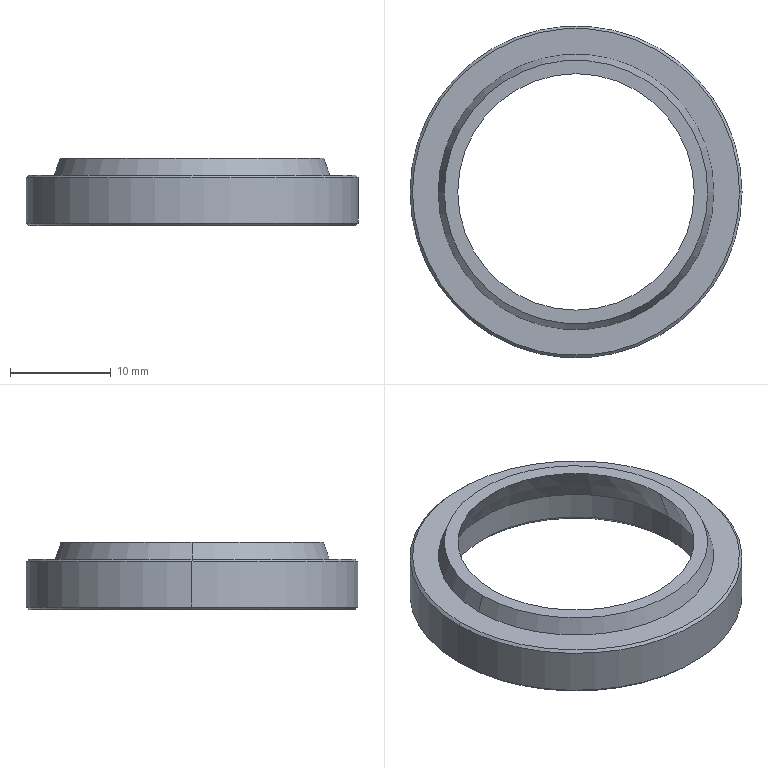Part | STEP file | Dust seal DHS25×33×4.5 | 1 solid | 17 faces | box 33 x 33 x 6.667 mm | volume 1830 mm3 | cone 10 | cylinder 4 | plane 3 | commonest cylinder face diameters 26 x2 33 x2
STEP:
#1=CARTESIAN_POINT('',(0.,0.,0.));
#2=DIRECTION('',(0.,0.,1.));
#3=DIRECTION('',(1.,0.,0.));
#4=AXIS2_PLACEMENT_3D('',#1,#2,#3);
#5=CARTESIAN_POINT('',(-16.25,0.,-6.667));
#6=VERTEX_POINT('',#5);
#7=CARTESIAN_POINT('',(16.25,0.,-6.667));
#8=VERTEX_POINT('',#7);
#9=CARTESIAN_POINT('',(0.,0.,-6.667));
#10=DIRECTION('',(0.,0.,-1.));
#11=DIRECTION('',(1.,0.,0.));
#12=AXIS2_PLACEMENT_3D('',#9,#10,#11);
#13=CIRCLE('',#12,16.25);
#14=CARTESIAN_POINT('',(0.,0.,-6.417));
#15=DIRECTION('',(0.,0.,1.));
#16=DIRECTION('',(1.,0.,0.));
#17=AXIS2_PLACEMENT_3D('',#14,#15,#16);
#18=CONICAL_SURFACE('',#17,16.5,0.7854);
#19=CARTESIAN_POINT('',(6.283,-0.25));
#20=DIRECTION('',(-1.,0.));
#21=VECTOR('',#20,1.);
#22=LINE('',#19,#21);
#23=(GEOMETRIC_REPRESENTATION_CONTEXT(2)PARAMETRIC_REPRESENTATION_CONTEXT()REPRESENTATION_CONTEXT('',''));
#24=DEFINITIONAL_REPRESENTATION('',(#22),#23);
#25=PCURVE('',#18,#24);
#26=CARTESIAN_POINT('',(-13.,0.,-6.667));
#27=DIRECTION('',(0.,0.,1.));
#28=DIRECTION('',(1.,0.,0.));
#29=AXIS2_PLACEMENT_3D('',#26,#27,#28);
#30=PLANE('',#29);
#31=CARTESIAN_POINT('',(29.25,0.));
#32=CARTESIAN_POINT('',(29.25,-28.146));
#33=CARTESIAN_POINT('',(4.875,-14.073));
#34=CARTESIAN_POINT('',(-19.5,0.));
#35=CARTESIAN_POINT('',(4.875,14.073));
#36=CARTESIAN_POINT('',(29.25,28.146));
#37=CARTESIAN_POINT('',(29.25,0.));
#38=(BOUNDED_CURVE()B_SPLINE_CURVE(2,(#31,#32,#33,#34,#35,#36,#37),.UNSPECIFIED.,.T.,.F.)B_SPLINE_CURVE_WITH_KNOTS((1,2,2,2,2,1),(-2.094,0.,2.094,4.189,6.283,8.378),.UNSPECIFIED.)CURVE()GEOMETRIC_REPRESENTATION_ITEM()RATIONAL_B_SPLINE_CURVE((1.,0.5,1.,0.5,1.,0.5,1.))REPRESENTATION_ITEM(''));
#39=(GEOMETRIC_REPRESENTATION_CONTEXT(2)PARAMETRIC_REPRESENTATION_CONTEXT()REPRESENTATION_CONTEXT('',''));
#40=DEFINITIONAL_REPRESENTATION('',(#38),#39);
#41=PCURVE('',#30,#40);
#42=SURFACE_CURVE('',#13,(#25,#41),.PCURVE_S1.);
#43=EDGE_CURVE('',#6,#8,#42,.T.);
#44=ORIENTED_EDGE('',*,*,#43,.F.);
#45=CARTESIAN_POINT('',(-16.5,0.,-6.417));
#46=VERTEX_POINT('',#45);
#47=CARTESIAN_POINT('',(-16.5,0.,-6.417));
#48=DIRECTION('',(-0.7071,0.,0.7071));
#49=VECTOR('',#48,1.);
#50=LINE('',#47,#49);
#51=CARTESIAN_POINT('',(3.142,0.));
#52=DIRECTION('',(0.,1.));
#53=VECTOR('',#52,1.);
#54=LINE('',#51,#53);
#55=(GEOMETRIC_REPRESENTATION_CONTEXT(2)PARAMETRIC_REPRESENTATION_CONTEXT()REPRESENTATION_CONTEXT('',''));
#56=DEFINITIONAL_REPRESENTATION('',(#54),#55);
#57=PCURVE('',#18,#56);
#58=CARTESIAN_POINT('',(0.,0.,-6.417));
#59=DIRECTION('',(0.,0.,1.));
#60=DIRECTION('',(1.,0.,0.));
#61=AXIS2_PLACEMENT_3D('',#58,#59,#60);
#62=CONICAL_SURFACE('',#61,16.5,0.7854);
#63=CARTESIAN_POINT('',(3.142,0.));
#64=DIRECTION('',(0.,1.));
#65=VECTOR('',#64,1.);
#66=LINE('',#63,#65);
#67=(GEOMETRIC_REPRESENTATION_CONTEXT(2)PARAMETRIC_REPRESENTATION_CONTEXT()REPRESENTATION_CONTEXT('',''));
#68=DEFINITIONAL_REPRESENTATION('',(#66),#67);
#69=PCURVE('',#62,#68);
#70=SURFACE_CURVE('',#50,(#57,#69),.PCURVE_S1.);
#71=EDGE_CURVE('',#6,#46,#70,.T.);
#72=ORIENTED_EDGE('',*,*,#71,.T.);
#73=CARTESIAN_POINT('',(16.5,0.,-6.417));
#74=VERTEX_POINT('',#73);
#75=CARTESIAN_POINT('',(0.,0.,-6.417));
#76=DIRECTION('',(0.,0.,1.));
#77=DIRECTION('',(1.,0.,0.));
#78=AXIS2_PLACEMENT_3D('',#75,#76,#77);
#79=CIRCLE('',#78,16.5);
#80=CARTESIAN_POINT('',(0.,0.));
#81=DIRECTION('',(1.,0.));
#82=VECTOR('',#81,1.);
#83=LINE('',#80,#82);
#84=(GEOMETRIC_REPRESENTATION_CONTEXT(2)PARAMETRIC_REPRESENTATION_CONTEXT()REPRESENTATION_CONTEXT('',''));
#85=DEFINITIONAL_REPRESENTATION('',(#83),#84);
#86=PCURVE('',#18,#85);
#87=CARTESIAN_POINT('',(0.,0.,9.196));
#88=DIRECTION('',(0.,0.,1.));
#89=DIRECTION('',(1.,0.,0.));
#90=AXIS2_PLACEMENT_3D('',#87,#88,#89);
#91=CYLINDRICAL_SURFACE('',#90,16.5);
#92=CARTESIAN_POINT('',(0.,-15.613));
#93=DIRECTION('',(1.,0.));
#94=VECTOR('',#93,1.);
#95=LINE('',#92,#94);
#96=(GEOMETRIC_REPRESENTATION_CONTEXT(2)PARAMETRIC_REPRESENTATION_CONTEXT()REPRESENTATION_CONTEXT('',''));
#97=DEFINITIONAL_REPRESENTATION('',(#95),#96);
#98=PCURVE('',#91,#97);
#99=SURFACE_CURVE('',#79,(#86,#98),.PCURVE_S1.);
#100=EDGE_CURVE('',#74,#46,#99,.T.);
#101=ORIENTED_EDGE('',*,*,#100,.F.);
#102=CARTESIAN_POINT('',(16.5,0.,-6.417));
#103=DIRECTION('',(0.7071,0.,0.7071));
#104=VECTOR('',#103,1.);
#105=LINE('',#102,#104);
#106=CARTESIAN_POINT('',(0.,0.));
#107=DIRECTION('',(0.,1.));
#108=VECTOR('',#107,1.);
#109=LINE('',#106,#108);
#110=(GEOMETRIC_REPRESENTATION_CONTEXT(2)PARAMETRIC_REPRESENTATION_CONTEXT()REPRESENTATION_CONTEXT('',''));
#111=DEFINITIONAL_REPRESENTATION('',(#109),#110);
#112=PCURVE('',#18,#111);
#113=CARTESIAN_POINT('',(6.283,0.));
#114=DIRECTION('',(0.,1.));
#115=VECTOR('',#114,1.);
#116=LINE('',#113,#115);
#117=(GEOMETRIC_REPRESENTATION_CONTEXT(2)PARAMETRIC_REPRESENTATION_CONTEXT()REPRESENTATION_CONTEXT('',''));
#118=DEFINITIONAL_REPRESENTATION('',(#116),#117);
#119=PCURVE('',#62,#118);
#120=SURFACE_CURVE('',#105,(#112,#119),.PCURVE_S1.);
#121=EDGE_CURVE('',#8,#74,#120,.T.);
#122=ORIENTED_EDGE('',*,*,#121,.F.);
#123=EDGE_LOOP('',(#44,#72,#101,#122));
#124=FACE_BOUND('',#123,.T.);
#125=ADVANCED_FACE('',(#124),#18,.T.);
#126=CARTESIAN_POINT('',(16.25,0.,-1.667));
#127=VERTEX_POINT('',#126);
#128=CARTESIAN_POINT('',(-16.25,0.,-1.667));
#129=VERTEX_POINT('',#128);
#130=CARTESIAN_POINT('',(0.,0.,-1.667));
#131=DIRECTION('',(0.,0.,1.));
#132=DIRECTION('',(-1.,0.,0.));
#133=AXIS2_PLACEMENT_3D('',#130,#131,#132);
#134=CIRCLE('',#133,16.25);
#135=CARTESIAN_POINT('',(0.,0.,-1.667));
#136=DIRECTION('',(0.,0.,-1.));
#137=DIRECTION('',(-1.,0.,0.));
#138=AXIS2_PLACEMENT_3D('',#135,#136,#137);
#139=CONICAL_SURFACE('',#138,16.25,0.7854);
#140=CARTESIAN_POINT('',(6.283,0.));
#141=DIRECTION('',(-1.,0.));
#142=VECTOR('',#141,1.);
#143=LINE('',#140,#142);
#144=(GEOMETRIC_REPRESENTATION_CONTEXT(2)PARAMETRIC_REPRESENTATION_CONTEXT()REPRESENTATION_CONTEXT('',''));
#145=DEFINITIONAL_REPRESENTATION('',(#143),#144);
#146=PCURVE('',#139,#145);
#147=CARTESIAN_POINT('',(-13.7,0.,-1.667));
#148=DIRECTION('',(0.,0.,-1.));
#149=DIRECTION('',(-1.,0.,0.));
#150=AXIS2_PLACEMENT_3D('',#147,#148,#149);
#151=PLANE('',#150);
#152=CARTESIAN_POINT('',(2.55,0.));
#153=CARTESIAN_POINT('',(2.55,-28.146));
#154=CARTESIAN_POINT('',(-21.825,-14.073));
#155=CARTESIAN_POINT('',(-46.2,0.));
#156=CARTESIAN_POINT('',(-21.825,14.073));
#157=CARTESIAN_POINT('',(2.55,28.146));
#158=CARTESIAN_POINT('',(2.55,0.));
#159=(BOUNDED_CURVE()B_SPLINE_CURVE(2,(#152,#153,#154,#155,#156,#157,#158),.UNSPECIFIED.,.T.,.F.)B_SPLINE_CURVE_WITH_KNOTS((1,2,2,2,2,1),(-2.094,0.,2.094,4.189,6.283,8.378),.UNSPECIFIED.)CURVE()GEOMETRIC_REPRESENTATION_ITEM()RATIONAL_B_SPLINE_CURVE((1.,0.5,1.,0.5,1.,0.5,1.))REPRESENTATION_ITEM(''));
#160=(GEOMETRIC_REPRESENTATION_CONTEXT(2)PARAMETRIC_REPRESENTATION_CONTEXT()REPRESENTATION_CONTEXT('',''));
#161=DEFINITIONAL_REPRESENTATION('',(#159),#160);
#162=PCURVE('',#151,#161);
#163=SURFACE_CURVE('',#134,(#146,#162),.PCURVE_S1.);
#164=EDGE_CURVE('',#127,#129,#163,.T.);
#165=ORIENTED_EDGE('',*,*,#164,.F.);
#166=CARTESIAN_POINT('',(16.5,0.,-1.917));
#167=VERTEX_POINT('',#166);
#168=CARTESIAN_POINT('',(16.25,0.,-1.667));
#169=DIRECTION('',(0.7071,0.,-0.7071));
#170=VECTOR('',#169,1.);
#171=LINE('',#168,#170);
#172=CARTESIAN_POINT('',(3.142,0.));
#173=DIRECTION('',(0.,1.));
#174=VECTOR('',#173,1.);
#175=LINE('',#172,#174);
#176=(GEOMETRIC_REPRESENTATION_CONTEXT(2)PARAMETRIC_REPRESENTATION_CONTEXT()REPRESENTATION_CONTEXT('',''));
#177=DEFINITIONAL_REPRESENTATION('',(#175),#176);
#178=PCURVE('',#139,#177);
#179=CARTESIAN_POINT('',(0.,0.,-1.667));
#180=DIRECTION('',(0.,0.,-1.));
#181=DIRECTION('',(-1.,0.,0.));
#182=AXIS2_PLACEMENT_3D('',#179,#180,#181);
#183=CONICAL_SURFACE('',#182,16.25,0.7854);
#184=CARTESIAN_POINT('',(3.142,0.));
#185=DIRECTION('',(0.,1.));
#186=VECTOR('',#185,1.);
#187=LINE('',#184,#186);
#188=(GEOMETRIC_REPRESENTATION_CONTEXT(2)PARAMETRIC_REPRESENTATION_CONTEXT()REPRESENTATION_CONTEXT('',''));
#189=DEFINITIONAL_REPRESENTATION('',(#187),#188);
#190=PCURVE('',#183,#189);
#191=SURFACE_CURVE('',#171,(#178,#190),.PCURVE_S1.);
#192=EDGE_CURVE('',#127,#167,#191,.T.);
#193=ORIENTED_EDGE('',*,*,#192,.T.);
#194=CARTESIAN_POINT('',(-16.5,0.,-1.917));
#195=VERTEX_POINT('',#194);
#196=CARTESIAN_POINT('',(0.,0.,-1.917));
#197=DIRECTION('',(0.,0.,-1.));
#198=DIRECTION('',(-1.,0.,0.));
#199=AXIS2_PLACEMENT_3D('',#196,#197,#198);
#200=CIRCLE('',#199,16.5);
#201=CARTESIAN_POINT('',(0.,0.25));
#202=DIRECTION('',(1.,0.));
#203=VECTOR('',#202,1.);
#204=LINE('',#201,#203);
#205=(GEOMETRIC_REPRESENTATION_CONTEXT(2)PARAMETRIC_REPRESENTATION_CONTEXT()REPRESENTATION_CONTEXT('',''));
#206=DEFINITIONAL_REPRESENTATION('',(#204),#205);
#207=PCURVE('',#139,#206);
#208=CARTESIAN_POINT('',(3.142,-11.113));
#209=DIRECTION('',(-1.,0.));
#210=VECTOR('',#209,1.);
#211=LINE('',#208,#210);
#212=(GEOMETRIC_REPRESENTATION_CONTEXT(2)PARAMETRIC_REPRESENTATION_CONTEXT()REPRESENTATION_CONTEXT('',''));
#213=DEFINITIONAL_REPRESENTATION('',(#211),#212);
#214=PCURVE('',#91,#213);
#215=SURFACE_CURVE('',#200,(#207,#214),.PCURVE_S1.);
#216=EDGE_CURVE('',#195,#167,#215,.T.);
#217=ORIENTED_EDGE('',*,*,#216,.F.);
#218=CARTESIAN_POINT('',(-16.25,0.,-1.667));
#219=DIRECTION('',(-0.7071,0.,-0.7071));
#220=VECTOR('',#219,1.);
#221=LINE('',#218,#220);
#222=CARTESIAN_POINT('',(0.,0.));
#223=DIRECTION('',(0.,1.));
#224=VECTOR('',#223,1.);
#225=LINE('',#222,#224);
#226=(GEOMETRIC_REPRESENTATION_CONTEXT(2)PARAMETRIC_REPRESENTATION_CONTEXT()REPRESENTATION_CONTEXT('',''));
#227=DEFINITIONAL_REPRESENTATION('',(#225),#226);
#228=PCURVE('',#139,#227);
#229=CARTESIAN_POINT('',(6.283,0.));
#230=DIRECTION('',(0.,1.));
#231=VECTOR('',#230,1.);
#232=LINE('',#229,#231);
#233=(GEOMETRIC_REPRESENTATION_CONTEXT(2)PARAMETRIC_REPRESENTATION_CONTEXT()REPRESENTATION_CONTEXT('',''));
#234=DEFINITIONAL_REPRESENTATION('',(#232),#233);
#235=PCURVE('',#183,#234);
#236=SURFACE_CURVE('',#221,(#228,#235),.PCURVE_S1.);
#237=EDGE_CURVE('',#129,#195,#236,.T.);
#238=ORIENTED_EDGE('',*,*,#237,.F.);
#239=EDGE_LOOP('',(#165,#193,#217,#238));
#240=FACE_BOUND('',#239,.T.);
#241=ADVANCED_FACE('',(#240),#139,.T.);
#242=CARTESIAN_POINT('',(-13.,0.,-6.167));
#243=VERTEX_POINT('',#242);
#244=CARTESIAN_POINT('',(-13.5,0.,-6.667));
#245=VERTEX_POINT('',#244);
#246=CARTESIAN_POINT('',(-13.5,0.,-6.667));
#247=DIRECTION('',(-0.7071,0.,-0.7071));
#248=VECTOR('',#247,1.);
#249=LINE('',#246,#248);
#250=CARTESIAN_POINT('',(0.,0.,-6.667));
#251=DIRECTION('',(0.,0.,-1.));
#252=DIRECTION('',(-1.,0.,0.));
#253=AXIS2_PLACEMENT_3D('',#250,#251,#252);
#254=CONICAL_SURFACE('',#253,13.5,0.7854);
#255=CARTESIAN_POINT('',(6.283,0.));
#256=DIRECTION('',(0.,1.));
#257=VECTOR('',#256,1.);
#258=LINE('',#255,#257);
#259=(GEOMETRIC_REPRESENTATION_CONTEXT(2)PARAMETRIC_REPRESENTATION_CONTEXT()REPRESENTATION_CONTEXT('',''));
#260=DEFINITIONAL_REPRESENTATION('',(#258),#259);
#261=PCURVE('',#254,#260);
#262=CARTESIAN_POINT('',(0.,0.,-6.667));
#263=DIRECTION('',(0.,0.,-1.));
#264=DIRECTION('',(-1.,0.,0.));
#265=AXIS2_PLACEMENT_3D('',#262,#263,#264);
#266=CONICAL_SURFACE('',#265,13.5,0.7854);
#267=CARTESIAN_POINT('',(0.,0.));
#268=DIRECTION('',(0.,1.));
#269=VECTOR('',#268,1.);
#270=LINE('',#267,#269);
#271=(GEOMETRIC_REPRESENTATION_CONTEXT(2)PARAMETRIC_REPRESENTATION_CONTEXT()REPRESENTATION_CONTEXT('',''));
#272=DEFINITIONAL_REPRESENTATION('',(#270),#271);
#273=PCURVE('',#266,#272);
#274=SURFACE_CURVE('',#249,(#261,#273),.PCURVE_S1.);
#275=EDGE_CURVE('',#243,#245,#274,.T.);
#276=ORIENTED_EDGE('',*,*,#275,.T.);
#277=CARTESIAN_POINT('',(13.5,0.,-6.667));
#278=VERTEX_POINT('',#277);
#279=CARTESIAN_POINT('',(0.,0.,-6.667));
#280=DIRECTION('',(0.,0.,1.));
#281=DIRECTION('',(1.,0.,0.));
#282=AXIS2_PLACEMENT_3D('',#279,#280,#281);
#283=CIRCLE('',#282,13.5);
#284=CARTESIAN_POINT('',(9.425,0.));
#285=DIRECTION('',(-1.,0.));
#286=VECTOR('',#285,1.);
#287=LINE('',#284,#286);
#288=(GEOMETRIC_REPRESENTATION_CONTEXT(2)PARAMETRIC_REPRESENTATION_CONTEXT()REPRESENTATION_CONTEXT('',''));
#289=DEFINITIONAL_REPRESENTATION('',(#287),#288);
#290=PCURVE('',#254,#289);
#291=CARTESIAN_POINT('',(13.,0.));
#292=DIRECTION('',(1.,0.));
#293=AXIS2_PLACEMENT_2D('',#291,#292);
#294=CIRCLE('',#293,13.5);
#295=(GEOMETRIC_REPRESENTATION_CONTEXT(2)PARAMETRIC_REPRESENTATION_CONTEXT()REPRESENTATION_CONTEXT('',''));
#296=DEFINITIONAL_REPRESENTATION('',(#294),#295);
#297=PCURVE('',#30,#296);
#298=SURFACE_CURVE('',#283,(#290,#297),.PCURVE_S1.);
#299=EDGE_CURVE('',#245,#278,#298,.T.);
#300=ORIENTED_EDGE('',*,*,#299,.T.);
#301=CARTESIAN_POINT('',(13.,0.,-6.167));
#302=VERTEX_POINT('',#301);
#303=CARTESIAN_POINT('',(13.5,0.,-6.667));
#304=DIRECTION('',(0.7071,0.,-0.7071));
#305=VECTOR('',#304,1.);
#306=LINE('',#303,#305);
#307=CARTESIAN_POINT('',(3.142,0.));
#308=DIRECTION('',(0.,1.));
#309=VECTOR('',#308,1.);
#310=LINE('',#307,#309);
#311=(GEOMETRIC_REPRESENTATION_CONTEXT(2)PARAMETRIC_REPRESENTATION_CONTEXT()REPRESENTATION_CONTEXT('',''));
#312=DEFINITIONAL_REPRESENTATION('',(#310),#311);
#313=PCURVE('',#254,#312);
#314=CARTESIAN_POINT('',(3.142,0.));
#315=DIRECTION('',(0.,1.));
#316=VECTOR('',#315,1.);
#317=LINE('',#314,#316);
#318=(GEOMETRIC_REPRESENTATION_CONTEXT(2)PARAMETRIC_REPRESENTATION_CONTEXT()REPRESENTATION_CONTEXT('',''));
#319=DEFINITIONAL_REPRESENTATION('',(#317),#318);
#320=PCURVE('',#266,#319);
#321=SURFACE_CURVE('',#306,(#313,#320),.PCURVE_S1.);
#322=EDGE_CURVE('',#302,#278,#321,.T.);
#323=ORIENTED_EDGE('',*,*,#322,.F.);
#324=CARTESIAN_POINT('',(0.,0.,-6.167));
#325=DIRECTION('',(0.,0.,-1.));
#326=DIRECTION('',(1.,0.,0.));
#327=AXIS2_PLACEMENT_3D('',#324,#325,#326);
#328=CIRCLE('',#327,13.);
#329=CARTESIAN_POINT('',(3.142,-0.5));
#330=DIRECTION('',(1.,0.));
#331=VECTOR('',#330,1.);
#332=LINE('',#329,#331);
#333=(GEOMETRIC_REPRESENTATION_CONTEXT(2)PARAMETRIC_REPRESENTATION_CONTEXT()REPRESENTATION_CONTEXT('',''));
#334=DEFINITIONAL_REPRESENTATION('',(#332),#333);
#335=PCURVE('',#254,#334);
#336=CARTESIAN_POINT('',(0.,0.,9.196));
#337=DIRECTION('',(0.,0.,1.));
#338=DIRECTION('',(1.,0.,0.));
#339=AXIS2_PLACEMENT_3D('',#336,#337,#338);
#340=CYLINDRICAL_SURFACE('',#339,13.);
#341=CARTESIAN_POINT('',(6.283,-15.363));
#342=DIRECTION('',(-1.,0.));
#343=VECTOR('',#342,1.);
#344=LINE('',#341,#343);
#345=(GEOMETRIC_REPRESENTATION_CONTEXT(2)PARAMETRIC_REPRESENTATION_CONTEXT()REPRESENTATION_CONTEXT('',''));
#346=DEFINITIONAL_REPRESENTATION('',(#344),#345);
#347=PCURVE('',#340,#346);
#348=SURFACE_CURVE('',#328,(#335,#347),.PCURVE_S1.);
#349=EDGE_CURVE('',#302,#243,#348,.T.);
#350=ORIENTED_EDGE('',*,*,#349,.T.);
#351=EDGE_LOOP('',(#276,#300,#323,#350));
#352=FACE_BOUND('',#351,.F.);
#353=ADVANCED_FACE('',(#352),#254,.F.);
#354=CARTESIAN_POINT('',(13.,0.,-3.434));
#355=VERTEX_POINT('',#354);
#356=CARTESIAN_POINT('',(13.,0.,9.196));
#357=DIRECTION('',(0.,0.,1.));
#358=VECTOR('',#357,1.);
#359=LINE('',#356,#358);
#360=CARTESIAN_POINT('',(6.283,0.));
#361=DIRECTION('',(0.,1.));
#362=VECTOR('',#361,1.);
#363=LINE('',#360,#362);
#364=(GEOMETRIC_REPRESENTATION_CONTEXT(2)PARAMETRIC_REPRESENTATION_CONTEXT()REPRESENTATION_CONTEXT('',''));
#365=DEFINITIONAL_REPRESENTATION('',(#363),#364);
#366=PCURVE('',#340,#365);
#367=CARTESIAN_POINT('',(0.,0.,9.196));
#368=DIRECTION('',(0.,0.,1.));
#369=DIRECTION('',(1.,0.,0.));
#370=AXIS2_PLACEMENT_3D('',#367,#368,#369);
#371=CYLINDRICAL_SURFACE('',#370,13.);
#372=CARTESIAN_POINT('',(0.,0.));
#373=DIRECTION('',(0.,1.));
#374=VECTOR('',#373,1.);
#375=LINE('',#372,#374);
#376=(GEOMETRIC_REPRESENTATION_CONTEXT(2)PARAMETRIC_REPRESENTATION_CONTEXT()REPRESENTATION_CONTEXT('',''));
#377=DEFINITIONAL_REPRESENTATION('',(#375),#376);
#378=PCURVE('',#371,#377);
#379=SURFACE_CURVE('',#359,(#366,#378),.PCURVE_S1.);
#380=EDGE_CURVE('',#302,#355,#379,.T.);
#381=ORIENTED_EDGE('',*,*,#380,.T.);
#382=CARTESIAN_POINT('',(-13.,0.,-3.434));
#383=VERTEX_POINT('',#382);
#384=CARTESIAN_POINT('',(0.,0.,-3.434));
#385=DIRECTION('',(0.,0.,1.));
#386=DIRECTION('',(1.,0.,0.));
#387=AXIS2_PLACEMENT_3D('',#384,#385,#386);
#388=CIRCLE('',#387,13.);
#389=CARTESIAN_POINT('',(0.,-12.63));
#390=DIRECTION('',(1.,0.));
#391=VECTOR('',#390,1.);
#392=LINE('',#389,#391);
#393=(GEOMETRIC_REPRESENTATION_CONTEXT(2)PARAMETRIC_REPRESENTATION_CONTEXT()REPRESENTATION_CONTEXT('',''));
#394=DEFINITIONAL_REPRESENTATION('',(#392),#393);
#395=PCURVE('',#340,#394);
#396=CARTESIAN_POINT('',(0.,0.,0.));
#397=DIRECTION('',(0.,0.,-1.));
#398=DIRECTION('',(-1.,0.,0.));
#399=AXIS2_PLACEMENT_3D('',#396,#397,#398);
#400=CONICAL_SURFACE('',#399,11.75,0.3491);
#401=CARTESIAN_POINT('',(9.425,3.434));
#402=DIRECTION('',(-1.,0.));
#403=VECTOR('',#402,1.);
#404=LINE('',#401,#403);
#405=(GEOMETRIC_REPRESENTATION_CONTEXT(2)PARAMETRIC_REPRESENTATION_CONTEXT()REPRESENTATION_CONTEXT('',''));
#406=DEFINITIONAL_REPRESENTATION('',(#404),#405);
#407=PCURVE('',#400,#406);
#408=SURFACE_CURVE('',#388,(#395,#407),.PCURVE_S1.);
#409=EDGE_CURVE('',#383,#355,#408,.T.);
#410=ORIENTED_EDGE('',*,*,#409,.F.);
#411=CARTESIAN_POINT('',(-13.,0.,9.196));
#412=DIRECTION('',(0.,0.,1.));
#413=VECTOR('',#412,1.);
#414=LINE('',#411,#413);
#415=CARTESIAN_POINT('',(3.142,0.));
#416=DIRECTION('',(0.,1.));
#417=VECTOR('',#416,1.);
#418=LINE('',#415,#417);
#419=(GEOMETRIC_REPRESENTATION_CONTEXT(2)PARAMETRIC_REPRESENTATION_CONTEXT()REPRESENTATION_CONTEXT('',''));
#420=DEFINITIONAL_REPRESENTATION('',(#418),#419);
#421=PCURVE('',#340,#420);
#422=CARTESIAN_POINT('',(3.142,0.));
#423=DIRECTION('',(0.,1.));
#424=VECTOR('',#423,1.);
#425=LINE('',#422,#424);
#426=(GEOMETRIC_REPRESENTATION_CONTEXT(2)PARAMETRIC_REPRESENTATION_CONTEXT()REPRESENTATION_CONTEXT('',''));
#427=DEFINITIONAL_REPRESENTATION('',(#425),#426);
#428=PCURVE('',#371,#427);
#429=SURFACE_CURVE('',#414,(#421,#428),.PCURVE_S1.);
#430=EDGE_CURVE('',#243,#383,#429,.T.);
#431=ORIENTED_EDGE('',*,*,#430,.F.);
#432=ORIENTED_EDGE('',*,*,#349,.F.);
#433=EDGE_LOOP('',(#381,#410,#431,#432));
#434=FACE_BOUND('',#433,.F.);
#435=ADVANCED_FACE('',(#434),#340,.F.);
#436=CARTESIAN_POINT('',(-11.75,0.,0.));
#437=VERTEX_POINT('',#436);
#438=CARTESIAN_POINT('',(-11.75,0.,0.));
#439=DIRECTION('',(-0.342,0.,-0.9397));
#440=VECTOR('',#439,1.);
#441=LINE('',#438,#440);
#442=CARTESIAN_POINT('',(6.283,0.));
#443=DIRECTION('',(0.,1.));
#444=VECTOR('',#443,1.);
#445=LINE('',#442,#444);
#446=(GEOMETRIC_REPRESENTATION_CONTEXT(2)PARAMETRIC_REPRESENTATION_CONTEXT()REPRESENTATION_CONTEXT('',''));
#447=DEFINITIONAL_REPRESENTATION('',(#445),#446);
#448=PCURVE('',#400,#447);
#449=CARTESIAN_POINT('',(0.,0.,0.));
#450=DIRECTION('',(0.,0.,-1.));
#451=DIRECTION('',(-1.,0.,0.));
#452=AXIS2_PLACEMENT_3D('',#449,#450,#451);
#453=CONICAL_SURFACE('',#452,11.75,0.3491);
#454=CARTESIAN_POINT('',(0.,0.));
#455=DIRECTION('',(0.,1.));
#456=VECTOR('',#455,1.);
#457=LINE('',#454,#456);
#458=(GEOMETRIC_REPRESENTATION_CONTEXT(2)PARAMETRIC_REPRESENTATION_CONTEXT()REPRESENTATION_CONTEXT('',''));
#459=DEFINITIONAL_REPRESENTATION('',(#457),#458);
#460=PCURVE('',#453,#459);
#461=SURFACE_CURVE('',#441,(#448,#460),.PCURVE_S1.);
#462=EDGE_CURVE('',#437,#383,#461,.T.);
#463=ORIENTED_EDGE('',*,*,#462,.T.);
#464=ORIENTED_EDGE('',*,*,#409,.T.);
#465=CARTESIAN_POINT('',(11.75,0.,0.));
#466=VERTEX_POINT('',#465);
#467=CARTESIAN_POINT('',(11.75,0.,0.));
#468=DIRECTION('',(0.342,0.,-0.9397));
#469=VECTOR('',#468,1.);
#470=LINE('',#467,#469);
#471=CARTESIAN_POINT('',(3.142,0.));
#472=DIRECTION('',(0.,1.));
#473=VECTOR('',#472,1.);
#474=LINE('',#471,#473);
#475=(GEOMETRIC_REPRESENTATION_CONTEXT(2)PARAMETRIC_REPRESENTATION_CONTEXT()REPRESENTATION_CONTEXT('',''));
#476=DEFINITIONAL_REPRESENTATION('',(#474),#475);
#477=PCURVE('',#400,#476);
#478=CARTESIAN_POINT('',(3.142,0.));
#479=DIRECTION('',(0.,1.));
#480=VECTOR('',#479,1.);
#481=LINE('',#478,#480);
#482=(GEOMETRIC_REPRESENTATION_CONTEXT(2)PARAMETRIC_REPRESENTATION_CONTEXT()REPRESENTATION_CONTEXT('',''));
#483=DEFINITIONAL_REPRESENTATION('',(#481),#482);
#484=PCURVE('',#453,#483);
#485=SURFACE_CURVE('',#470,(#477,#484),.PCURVE_S1.);
#486=EDGE_CURVE('',#466,#355,#485,.T.);
#487=ORIENTED_EDGE('',*,*,#486,.F.);
#488=CARTESIAN_POINT('',(0.,0.,0.));
#489=DIRECTION('',(0.,0.,1.));
#490=DIRECTION('',(1.,0.,0.));
#491=AXIS2_PLACEMENT_3D('',#488,#489,#490);
#492=CIRCLE('',#491,11.75);
#493=CARTESIAN_POINT('',(9.425,0.));
#494=DIRECTION('',(-1.,0.));
#495=VECTOR('',#494,1.);
#496=LINE('',#493,#495);
#497=(GEOMETRIC_REPRESENTATION_CONTEXT(2)PARAMETRIC_REPRESENTATION_CONTEXT()REPRESENTATION_CONTEXT('',''));
#498=DEFINITIONAL_REPRESENTATION('',(#496),#497);
#499=PCURVE('',#400,#498);
#500=CARTESIAN_POINT('',(-11.75,0.,0.));
#501=DIRECTION('',(0.,0.,-1.));
#502=DIRECTION('',(-1.,0.,0.));
#503=AXIS2_PLACEMENT_3D('',#500,#501,#502);
#504=PLANE('',#503);
#505=CARTESIAN_POINT('',(-23.5,0.));
#506=CARTESIAN_POINT('',(-23.5,20.352));
#507=CARTESIAN_POINT('',(-5.875,10.176));
#508=CARTESIAN_POINT('',(11.75,0.));
#509=CARTESIAN_POINT('',(-5.875,-10.176));
#510=CARTESIAN_POINT('',(-23.5,-20.352));
#511=CARTESIAN_POINT('',(-23.5,0.));
#512=(BOUNDED_CURVE()B_SPLINE_CURVE(2,(#505,#506,#507,#508,#509,#510,#511),.UNSPECIFIED.,.T.,.F.)B_SPLINE_CURVE_WITH_KNOTS((1,2,2,2,2,1),(-2.094,0.,2.094,4.189,6.283,8.378),.UNSPECIFIED.)CURVE()GEOMETRIC_REPRESENTATION_ITEM()RATIONAL_B_SPLINE_CURVE((1.,0.5,1.,0.5,1.,0.5,1.))REPRESENTATION_ITEM(''));
#513=(GEOMETRIC_REPRESENTATION_CONTEXT(2)PARAMETRIC_REPRESENTATION_CONTEXT()REPRESENTATION_CONTEXT('',''));
#514=DEFINITIONAL_REPRESENTATION('',(#512),#513);
#515=PCURVE('',#504,#514);
#516=SURFACE_CURVE('',#492,(#499,#515),.PCURVE_S1.);
#517=EDGE_CURVE('',#437,#466,#516,.T.);
#518=ORIENTED_EDGE('',*,*,#517,.F.);
#519=EDGE_LOOP('',(#463,#464,#487,#518));
#520=FACE_BOUND('',#519,.F.);
#521=ADVANCED_FACE('',(#520),#400,.F.);
#522=CARTESIAN_POINT('',(13.093,0.,0.));
#523=VERTEX_POINT('',#522);
#524=CARTESIAN_POINT('',(-13.093,0.,0.));
#525=VERTEX_POINT('',#524);
#526=CARTESIAN_POINT('',(0.,0.,0.));
#527=DIRECTION('',(0.,0.,1.));
#528=DIRECTION('',(1.,0.,0.));
#529=AXIS2_PLACEMENT_3D('',#526,#527,#528);
#530=CIRCLE('',#529,13.093);
#531=CARTESIAN_POINT('',(0.,0.,-1.667));
#532=DIRECTION('',(0.,0.,-1.));
#533=DIRECTION('',(-1.,0.,0.));
#534=AXIS2_PLACEMENT_3D('',#531,#532,#533);
#535=CONICAL_SURFACE('',#534,13.7,0.3491);
#536=CARTESIAN_POINT('',(3.142,-1.667));
#537=DIRECTION('',(-1.,0.));
#538=VECTOR('',#537,1.);
#539=LINE('',#536,#538);
#540=(GEOMETRIC_REPRESENTATION_CONTEXT(2)PARAMETRIC_REPRESENTATION_CONTEXT()REPRESENTATION_CONTEXT('',''));
#541=DEFINITIONAL_REPRESENTATION('',(#539),#540);
#542=PCURVE('',#535,#541);
#543=CARTESIAN_POINT('',(-24.843,0.));
#544=CARTESIAN_POINT('',(-24.843,22.678));
#545=CARTESIAN_POINT('',(-5.203,11.339));
#546=CARTESIAN_POINT('',(14.437,0.));
#547=CARTESIAN_POINT('',(-5.203,-11.339));
#548=CARTESIAN_POINT('',(-24.843,-22.678));
#549=CARTESIAN_POINT('',(-24.843,0.));
#550=(BOUNDED_CURVE()B_SPLINE_CURVE(2,(#543,#544,#545,#546,#547,#548,#549),.UNSPECIFIED.,.T.,.F.)B_SPLINE_CURVE_WITH_KNOTS((1,2,2,2,2,1),(-2.094,0.,2.094,4.189,6.283,8.378),.UNSPECIFIED.)CURVE()GEOMETRIC_REPRESENTATION_ITEM()RATIONAL_B_SPLINE_CURVE((1.,0.5,1.,0.5,1.,0.5,1.))REPRESENTATION_ITEM(''));
#551=(GEOMETRIC_REPRESENTATION_CONTEXT(2)PARAMETRIC_REPRESENTATION_CONTEXT()REPRESENTATION_CONTEXT('',''));
#552=DEFINITIONAL_REPRESENTATION('',(#550),#551);
#553=PCURVE('',#504,#552);
#554=SURFACE_CURVE('',#530,(#542,#553),.PCURVE_S1.);
#555=EDGE_CURVE('',#523,#525,#554,.T.);
#556=ORIENTED_EDGE('',*,*,#555,.F.);
#557=CARTESIAN_POINT('',(13.7,0.,-1.667));
#558=VERTEX_POINT('',#557);
#559=CARTESIAN_POINT('',(13.7,0.,-1.667));
#560=DIRECTION('',(0.342,0.,-0.9397));
#561=VECTOR('',#560,1.);
#562=LINE('',#559,#561);
#563=CARTESIAN_POINT('',(3.142,0.));
#564=DIRECTION('',(0.,1.));
#565=VECTOR('',#564,1.);
#566=LINE('',#563,#565);
#567=(GEOMETRIC_REPRESENTATION_CONTEXT(2)PARAMETRIC_REPRESENTATION_CONTEXT()REPRESENTATION_CONTEXT('',''));
#568=DEFINITIONAL_REPRESENTATION('',(#566),#567);
#569=PCURVE('',#535,#568);
#570=CARTESIAN_POINT('',(0.,0.,-1.667));
#571=DIRECTION('',(0.,0.,-1.));
#572=DIRECTION('',(-1.,0.,0.));
#573=AXIS2_PLACEMENT_3D('',#570,#571,#572);
#574=CONICAL_SURFACE('',#573,13.7,0.3491);
#575=CARTESIAN_POINT('',(3.142,0.));
#576=DIRECTION('',(0.,1.));
#577=VECTOR('',#576,1.);
#578=LINE('',#575,#577);
#579=(GEOMETRIC_REPRESENTATION_CONTEXT(2)PARAMETRIC_REPRESENTATION_CONTEXT()REPRESENTATION_CONTEXT('',''));
#580=DEFINITIONAL_REPRESENTATION('',(#578),#579);
#581=PCURVE('',#574,#580);
#582=SURFACE_CURVE('',#562,(#569,#581),.PCURVE_S1.);
#583=EDGE_CURVE('',#523,#558,#582,.T.);
#584=ORIENTED_EDGE('',*,*,#583,.T.);
#585=CARTESIAN_POINT('',(-13.7,0.,-1.667));
#586=VERTEX_POINT('',#585);
#587=CARTESIAN_POINT('',(0.,0.,-1.667));
#588=DIRECTION('',(0.,0.,1.));
#589=DIRECTION('',(1.,0.,0.));
#590=AXIS2_PLACEMENT_3D('',#587,#588,#589);
#591=CIRCLE('',#590,13.7);
#592=CARTESIAN_POINT('',(3.142,0.));
#593=DIRECTION('',(-1.,0.));
#594=VECTOR('',#593,1.);
#595=LINE('',#592,#594);
#596=(GEOMETRIC_REPRESENTATION_CONTEXT(2)PARAMETRIC_REPRESENTATION_CONTEXT()REPRESENTATION_CONTEXT('',''));
#597=DEFINITIONAL_REPRESENTATION('',(#595),#596);
#598=PCURVE('',#535,#597);
#599=CARTESIAN_POINT('',(-27.4,0.));
#600=CARTESIAN_POINT('',(-27.4,23.729));
#601=CARTESIAN_POINT('',(-6.85,11.865));
#602=CARTESIAN_POINT('',(13.7,0.));
#603=CARTESIAN_POINT('',(-6.85,-11.865));
#604=CARTESIAN_POINT('',(-27.4,-23.729));
#605=CARTESIAN_POINT('',(-27.4,0.));
#606=(BOUNDED_CURVE()B_SPLINE_CURVE(2,(#599,#600,#601,#602,#603,#604,#605),.UNSPECIFIED.,.T.,.F.)B_SPLINE_CURVE_WITH_KNOTS((1,2,2,2,2,1),(-2.094,0.,2.094,4.189,6.283,8.378),.UNSPECIFIED.)CURVE()GEOMETRIC_REPRESENTATION_ITEM()RATIONAL_B_SPLINE_CURVE((1.,0.5,1.,0.5,1.,0.5,1.))REPRESENTATION_ITEM(''));
#607=(GEOMETRIC_REPRESENTATION_CONTEXT(2)PARAMETRIC_REPRESENTATION_CONTEXT()REPRESENTATION_CONTEXT('',''));
#608=DEFINITIONAL_REPRESENTATION('',(#606),#607);
#609=PCURVE('',#151,#608);
#610=SURFACE_CURVE('',#591,(#598,#609),.PCURVE_S1.);
#611=EDGE_CURVE('',#558,#586,#610,.T.);
#612=ORIENTED_EDGE('',*,*,#611,.T.);
#613=CARTESIAN_POINT('',(-13.7,0.,-1.667));
#614=DIRECTION('',(-0.342,0.,-0.9397));
#615=VECTOR('',#614,1.);
#616=LINE('',#613,#615);
#617=CARTESIAN_POINT('',(0.,0.));
#618=DIRECTION('',(0.,1.));
#619=VECTOR('',#618,1.);
#620=LINE('',#617,#619);
#621=(GEOMETRIC_REPRESENTATION_CONTEXT(2)PARAMETRIC_REPRESENTATION_CONTEXT()REPRESENTATION_CONTEXT('',''));
#622=DEFINITIONAL_REPRESENTATION('',(#620),#621);
#623=PCURVE('',#535,#622);
#624=CARTESIAN_POINT('',(6.283,0.));
#625=DIRECTION('',(0.,1.));
#626=VECTOR('',#625,1.);
#627=LINE('',#624,#626);
#628=(GEOMETRIC_REPRESENTATION_CONTEXT(2)PARAMETRIC_REPRESENTATION_CONTEXT()REPRESENTATION_CONTEXT('',''));
#629=DEFINITIONAL_REPRESENTATION('',(#627),#628);
#630=PCURVE('',#574,#629);
#631=SURFACE_CURVE('',#616,(#623,#630),.PCURVE_S1.);
#632=EDGE_CURVE('',#525,#586,#631,.T.);
#633=ORIENTED_EDGE('',*,*,#632,.F.);
#634=EDGE_LOOP('',(#556,#584,#612,#633));
#635=FACE_BOUND('',#634,.T.);
#636=ADVANCED_FACE('',(#635),#535,.T.);
#637=ORIENTED_EDGE('',*,*,#100,.T.);
#638=CARTESIAN_POINT('',(-16.5,0.,9.196));
#639=DIRECTION('',(0.,0.,1.));
#640=VECTOR('',#639,1.);
#641=LINE('',#638,#640);
#642=CARTESIAN_POINT('',(3.142,0.));
#643=DIRECTION('',(0.,1.));
#644=VECTOR('',#643,1.);
#645=LINE('',#642,#644);
#646=(GEOMETRIC_REPRESENTATION_CONTEXT(2)PARAMETRIC_REPRESENTATION_CONTEXT()REPRESENTATION_CONTEXT('',''));
#647=DEFINITIONAL_REPRESENTATION('',(#645),#646);
#648=PCURVE('',#91,#647);
#649=CARTESIAN_POINT('',(0.,0.,9.196));
#650=DIRECTION('',(0.,0.,1.));
#651=DIRECTION('',(1.,0.,0.));
#652=AXIS2_PLACEMENT_3D('',#649,#650,#651);
#653=CYLINDRICAL_SURFACE('',#652,16.5);
#654=CARTESIAN_POINT('',(3.142,0.));
#655=DIRECTION('',(0.,1.));
#656=VECTOR('',#655,1.);
#657=LINE('',#654,#656);
#658=(GEOMETRIC_REPRESENTATION_CONTEXT(2)PARAMETRIC_REPRESENTATION_CONTEXT()REPRESENTATION_CONTEXT('',''));
#659=DEFINITIONAL_REPRESENTATION('',(#657),#658);
#660=PCURVE('',#653,#659);
#661=SURFACE_CURVE('',#641,(#648,#660),.PCURVE_S1.);
#662=EDGE_CURVE('',#46,#195,#661,.T.);
#663=ORIENTED_EDGE('',*,*,#662,.T.);
#664=ORIENTED_EDGE('',*,*,#216,.T.);
#665=CARTESIAN_POINT('',(16.5,0.,9.196));
#666=DIRECTION('',(0.,0.,1.));
#667=VECTOR('',#666,1.);
#668=LINE('',#665,#667);
#669=CARTESIAN_POINT('',(0.,0.));
#670=DIRECTION('',(0.,1.));
#671=VECTOR('',#670,1.);
#672=LINE('',#669,#671);
#673=(GEOMETRIC_REPRESENTATION_CONTEXT(2)PARAMETRIC_REPRESENTATION_CONTEXT()REPRESENTATION_CONTEXT('',''));
#674=DEFINITIONAL_REPRESENTATION('',(#672),#673);
#675=PCURVE('',#91,#674);
#676=CARTESIAN_POINT('',(6.283,0.));
#677=DIRECTION('',(0.,1.));
#678=VECTOR('',#677,1.);
#679=LINE('',#676,#678);
#680=(GEOMETRIC_REPRESENTATION_CONTEXT(2)PARAMETRIC_REPRESENTATION_CONTEXT()REPRESENTATION_CONTEXT('',''));
#681=DEFINITIONAL_REPRESENTATION('',(#679),#680);
#682=PCURVE('',#653,#681);
#683=SURFACE_CURVE('',#668,(#675,#682),.PCURVE_S1.);
#684=EDGE_CURVE('',#74,#167,#683,.T.);
#685=ORIENTED_EDGE('',*,*,#684,.F.);
#686=EDGE_LOOP('',(#637,#663,#664,#685));
#687=FACE_BOUND('',#686,.T.);
#688=ADVANCED_FACE('',(#687),#91,.T.);
#689=CARTESIAN_POINT('',(0.,0.,-6.667));
#690=DIRECTION('',(0.,0.,-1.));
#691=DIRECTION('',(1.,0.,0.));
#692=AXIS2_PLACEMENT_3D('',#689,#690,#691);
#693=CIRCLE('',#692,16.25);
#694=CARTESIAN_POINT('',(29.25,0.));
#695=CARTESIAN_POINT('',(29.25,-28.146));
#696=CARTESIAN_POINT('',(4.875,-14.073));
#697=CARTESIAN_POINT('',(-19.5,0.));
#698=CARTESIAN_POINT('',(4.875,14.073));
#699=CARTESIAN_POINT('',(29.25,28.146));
#700=CARTESIAN_POINT('',(29.25,0.));
#701=(BOUNDED_CURVE()B_SPLINE_CURVE(2,(#694,#695,#696,#697,#698,#699,#700),.UNSPECIFIED.,.T.,.F.)B_SPLINE_CURVE_WITH_KNOTS((1,2,2,2,2,1),(-2.094,0.,2.094,4.189,6.283,8.378),.UNSPECIFIED.)CURVE()GEOMETRIC_REPRESENTATION_ITEM()RATIONAL_B_SPLINE_CURVE((1.,0.5,1.,0.5,1.,0.5,1.))REPRESENTATION_ITEM(''));
#702=(GEOMETRIC_REPRESENTATION_CONTEXT(2)PARAMETRIC_REPRESENTATION_CONTEXT()REPRESENTATION_CONTEXT('',''));
#703=DEFINITIONAL_REPRESENTATION('',(#701),#702);
#704=PCURVE('',#30,#703);
#705=CARTESIAN_POINT('',(6.283,-0.25));
#706=DIRECTION('',(-1.,0.));
#707=VECTOR('',#706,1.);
#708=LINE('',#705,#707);
#709=(GEOMETRIC_REPRESENTATION_CONTEXT(2)PARAMETRIC_REPRESENTATION_CONTEXT()REPRESENTATION_CONTEXT('',''));
#710=DEFINITIONAL_REPRESENTATION('',(#708),#709);
#711=PCURVE('',#62,#710);
#712=SURFACE_CURVE('',#693,(#704,#711),.PCURVE_S1.);
#713=EDGE_CURVE('',#8,#6,#712,.T.);
#714=ORIENTED_EDGE('',*,*,#713,.T.);
#715=ORIENTED_EDGE('',*,*,#43,.T.);
#716=EDGE_LOOP('',(#714,#715));
#717=FACE_BOUND('',#716,.T.);
#718=ORIENTED_EDGE('',*,*,#299,.T.);
#719=CARTESIAN_POINT('',(0.,0.,-6.667));
#720=DIRECTION('',(0.,0.,1.));
#721=DIRECTION('',(1.,0.,0.));
#722=AXIS2_PLACEMENT_3D('',#719,#720,#721);
#723=CIRCLE('',#722,13.5);
#724=CARTESIAN_POINT('',(13.,0.));
#725=DIRECTION('',(1.,0.));
#726=AXIS2_PLACEMENT_2D('',#724,#725);
#727=CIRCLE('',#726,13.5);
#728=(GEOMETRIC_REPRESENTATION_CONTEXT(2)PARAMETRIC_REPRESENTATION_CONTEXT()REPRESENTATION_CONTEXT('',''));
#729=DEFINITIONAL_REPRESENTATION('',(#727),#728);
#730=PCURVE('',#30,#729);
#731=CARTESIAN_POINT('',(3.142,0.));
#732=DIRECTION('',(-1.,0.));
#733=VECTOR('',#732,1.);
#734=LINE('',#731,#733);
#735=(GEOMETRIC_REPRESENTATION_CONTEXT(2)PARAMETRIC_REPRESENTATION_CONTEXT()REPRESENTATION_CONTEXT('',''));
#736=DEFINITIONAL_REPRESENTATION('',(#734),#735);
#737=PCURVE('',#266,#736);
#738=SURFACE_CURVE('',#723,(#730,#737),.PCURVE_S1.);
#739=EDGE_CURVE('',#278,#245,#738,.T.);
#740=ORIENTED_EDGE('',*,*,#739,.T.);
#741=EDGE_LOOP('',(#718,#740));
#742=FACE_BOUND('',#741,.T.);
#743=ADVANCED_FACE('',(#717,#742),#30,.F.);
#744=ORIENTED_EDGE('',*,*,#662,.F.);
#745=CARTESIAN_POINT('',(0.,0.,-6.417));
#746=DIRECTION('',(0.,0.,1.));
#747=DIRECTION('',(1.,0.,0.));
#748=AXIS2_PLACEMENT_3D('',#745,#746,#747);
#749=CIRCLE('',#748,16.5);
#750=CARTESIAN_POINT('',(0.,-15.613));
#751=DIRECTION('',(1.,0.));
#752=VECTOR('',#751,1.);
#753=LINE('',#750,#752);
#754=(GEOMETRIC_REPRESENTATION_CONTEXT(2)PARAMETRIC_REPRESENTATION_CONTEXT()REPRESENTATION_CONTEXT('',''));
#755=DEFINITIONAL_REPRESENTATION('',(#753),#754);
#756=PCURVE('',#653,#755);
#757=CARTESIAN_POINT('',(0.,0.));
#758=DIRECTION('',(1.,0.));
#759=VECTOR('',#758,1.);
#760=LINE('',#757,#759);
#761=(GEOMETRIC_REPRESENTATION_CONTEXT(2)PARAMETRIC_REPRESENTATION_CONTEXT()REPRESENTATION_CONTEXT('',''));
#762=DEFINITIONAL_REPRESENTATION('',(#760),#761);
#763=PCURVE('',#62,#762);
#764=SURFACE_CURVE('',#749,(#756,#763),.PCURVE_S1.);
#765=EDGE_CURVE('',#46,#74,#764,.T.);
#766=ORIENTED_EDGE('',*,*,#765,.T.);
#767=ORIENTED_EDGE('',*,*,#684,.T.);
#768=CARTESIAN_POINT('',(0.,0.,-1.917));
#769=DIRECTION('',(0.,0.,-1.));
#770=DIRECTION('',(-1.,0.,0.));
#771=AXIS2_PLACEMENT_3D('',#768,#769,#770);
#772=CIRCLE('',#771,16.5);
#773=CARTESIAN_POINT('',(9.425,-11.113));
#774=DIRECTION('',(-1.,0.));
#775=VECTOR('',#774,1.);
#776=LINE('',#773,#775);
#777=(GEOMETRIC_REPRESENTATION_CONTEXT(2)PARAMETRIC_REPRESENTATION_CONTEXT()REPRESENTATION_CONTEXT('',''));
#778=DEFINITIONAL_REPRESENTATION('',(#776),#777);
#779=PCURVE('',#653,#778);
#780=CARTESIAN_POINT('',(0.,0.25));
#781=DIRECTION('',(1.,0.));
#782=VECTOR('',#781,1.);
#783=LINE('',#780,#782);
#784=(GEOMETRIC_REPRESENTATION_CONTEXT(2)PARAMETRIC_REPRESENTATION_CONTEXT()REPRESENTATION_CONTEXT('',''));
#785=DEFINITIONAL_REPRESENTATION('',(#783),#784);
#786=PCURVE('',#183,#785);
#787=SURFACE_CURVE('',#772,(#779,#786),.PCURVE_S1.);
#788=EDGE_CURVE('',#167,#195,#787,.T.);
#789=ORIENTED_EDGE('',*,*,#788,.T.);
#790=EDGE_LOOP('',(#744,#766,#767,#789));
#791=FACE_BOUND('',#790,.T.);
#792=ADVANCED_FACE('',(#791),#653,.T.);
#793=CARTESIAN_POINT('',(0.,0.,-1.667));
#794=DIRECTION('',(0.,0.,1.));
#795=DIRECTION('',(-1.,0.,0.));
#796=AXIS2_PLACEMENT_3D('',#793,#794,#795);
#797=CIRCLE('',#796,16.25);
#798=CARTESIAN_POINT('',(2.55,0.));
#799=CARTESIAN_POINT('',(2.55,-28.146));
#800=CARTESIAN_POINT('',(-21.825,-14.073));
#801=CARTESIAN_POINT('',(-46.2,0.));
#802=CARTESIAN_POINT('',(-21.825,14.073));
#803=CARTESIAN_POINT('',(2.55,28.146));
#804=CARTESIAN_POINT('',(2.55,0.));
#805=(BOUNDED_CURVE()B_SPLINE_CURVE(2,(#798,#799,#800,#801,#802,#803,#804),.UNSPECIFIED.,.T.,.F.)B_SPLINE_CURVE_WITH_KNOTS((1,2,2,2,2,1),(-2.094,0.,2.094,4.189,6.283,8.378),.UNSPECIFIED.)CURVE()GEOMETRIC_REPRESENTATION_ITEM()RATIONAL_B_SPLINE_CURVE((1.,0.5,1.,0.5,1.,0.5,1.))REPRESENTATION_ITEM(''));
#806=(GEOMETRIC_REPRESENTATION_CONTEXT(2)PARAMETRIC_REPRESENTATION_CONTEXT()REPRESENTATION_CONTEXT('',''));
#807=DEFINITIONAL_REPRESENTATION('',(#805),#806);
#808=PCURVE('',#151,#807);
#809=CARTESIAN_POINT('',(6.283,0.));
#810=DIRECTION('',(-1.,0.));
#811=VECTOR('',#810,1.);
#812=LINE('',#809,#811);
#813=(GEOMETRIC_REPRESENTATION_CONTEXT(2)PARAMETRIC_REPRESENTATION_CONTEXT()REPRESENTATION_CONTEXT('',''));
#814=DEFINITIONAL_REPRESENTATION('',(#812),#813);
#815=PCURVE('',#183,#814);
#816=SURFACE_CURVE('',#797,(#808,#815),.PCURVE_S1.);
#817=EDGE_CURVE('',#129,#127,#816,.T.);
#818=ORIENTED_EDGE('',*,*,#817,.T.);
#819=ORIENTED_EDGE('',*,*,#164,.T.);
#820=EDGE_LOOP('',(#818,#819));
#821=FACE_BOUND('',#820,.T.);
#822=CARTESIAN_POINT('',(0.,0.,-1.667));
#823=DIRECTION('',(0.,0.,1.));
#824=DIRECTION('',(1.,0.,0.));
#825=AXIS2_PLACEMENT_3D('',#822,#823,#824);
#826=CIRCLE('',#825,13.7);
#827=CARTESIAN_POINT('',(-27.4,0.));
#828=CARTESIAN_POINT('',(-27.4,23.729));
#829=CARTESIAN_POINT('',(-6.85,11.865));
#830=CARTESIAN_POINT('',(13.7,0.));
#831=CARTESIAN_POINT('',(-6.85,-11.865));
#832=CARTESIAN_POINT('',(-27.4,-23.729));
#833=CARTESIAN_POINT('',(-27.4,0.));
#834=(BOUNDED_CURVE()B_SPLINE_CURVE(2,(#827,#828,#829,#830,#831,#832,#833),.UNSPECIFIED.,.T.,.F.)B_SPLINE_CURVE_WITH_KNOTS((1,2,2,2,2,1),(-2.094,0.,2.094,4.189,6.283,8.378),.UNSPECIFIED.)CURVE()GEOMETRIC_REPRESENTATION_ITEM()RATIONAL_B_SPLINE_CURVE((1.,0.5,1.,0.5,1.,0.5,1.))REPRESENTATION_ITEM(''));
#835=(GEOMETRIC_REPRESENTATION_CONTEXT(2)PARAMETRIC_REPRESENTATION_CONTEXT()REPRESENTATION_CONTEXT('',''));
#836=DEFINITIONAL_REPRESENTATION('',(#834),#835);
#837=PCURVE('',#151,#836);
#838=CARTESIAN_POINT('',(9.425,0.));
#839=DIRECTION('',(-1.,0.));
#840=VECTOR('',#839,1.);
#841=LINE('',#838,#840);
#842=(GEOMETRIC_REPRESENTATION_CONTEXT(2)PARAMETRIC_REPRESENTATION_CONTEXT()REPRESENTATION_CONTEXT('',''));
#843=DEFINITIONAL_REPRESENTATION('',(#841),#842);
#844=PCURVE('',#574,#843);
#845=SURFACE_CURVE('',#826,(#837,#844),.PCURVE_S1.);
#846=EDGE_CURVE('',#586,#558,#845,.T.);
#847=ORIENTED_EDGE('',*,*,#846,.F.);
#848=ORIENTED_EDGE('',*,*,#611,.F.);
#849=EDGE_LOOP('',(#847,#848));
#850=FACE_BOUND('',#849,.T.);
#851=ADVANCED_FACE('',(#821,#850),#151,.F.);
#852=ORIENTED_EDGE('',*,*,#583,.F.);
#853=CARTESIAN_POINT('',(0.,0.,0.));
#854=DIRECTION('',(0.,0.,1.));
#855=DIRECTION('',(1.,0.,0.));
#856=AXIS2_PLACEMENT_3D('',#853,#854,#855);
#857=CIRCLE('',#856,13.093);
#858=CARTESIAN_POINT('',(9.425,-1.667));
#859=DIRECTION('',(-1.,0.));
#860=VECTOR('',#859,1.);
#861=LINE('',#858,#860);
#862=(GEOMETRIC_REPRESENTATION_CONTEXT(2)PARAMETRIC_REPRESENTATION_CONTEXT()REPRESENTATION_CONTEXT('',''));
#863=DEFINITIONAL_REPRESENTATION('',(#861),#862);
#864=PCURVE('',#574,#863);
#865=CARTESIAN_POINT('',(-24.843,0.));
#866=CARTESIAN_POINT('',(-24.843,22.678));
#867=CARTESIAN_POINT('',(-5.203,11.339));
#868=CARTESIAN_POINT('',(14.437,0.));
#869=CARTESIAN_POINT('',(-5.203,-11.339));
#870=CARTESIAN_POINT('',(-24.843,-22.678));
#871=CARTESIAN_POINT('',(-24.843,0.));
#872=(BOUNDED_CURVE()B_SPLINE_CURVE(2,(#865,#866,#867,#868,#869,#870,#871),.UNSPECIFIED.,.T.,.F.)B_SPLINE_CURVE_WITH_KNOTS((1,2,2,2,2,1),(-2.094,0.,2.094,4.189,6.283,8.378),.UNSPECIFIED.)CURVE()GEOMETRIC_REPRESENTATION_ITEM()RATIONAL_B_SPLINE_CURVE((1.,0.5,1.,0.5,1.,0.5,1.))REPRESENTATION_ITEM(''));
#873=(GEOMETRIC_REPRESENTATION_CONTEXT(2)PARAMETRIC_REPRESENTATION_CONTEXT()REPRESENTATION_CONTEXT('',''));
#874=DEFINITIONAL_REPRESENTATION('',(#872),#873);
#875=PCURVE('',#504,#874);
#876=SURFACE_CURVE('',#857,(#864,#875),.PCURVE_S1.);
#877=EDGE_CURVE('',#525,#523,#876,.T.);
#878=ORIENTED_EDGE('',*,*,#877,.F.);
#879=ORIENTED_EDGE('',*,*,#632,.T.);
#880=ORIENTED_EDGE('',*,*,#846,.T.);
#881=EDGE_LOOP('',(#852,#878,#879,#880));
#882=FACE_BOUND('',#881,.T.);
#883=ADVANCED_FACE('',(#882),#574,.T.);
#884=ORIENTED_EDGE('',*,*,#517,.F.);
#885=CARTESIAN_POINT('',(0.,0.,0.));
#886=DIRECTION('',(0.,0.,1.));
#887=DIRECTION('',(1.,0.,0.));
#888=AXIS2_PLACEMENT_3D('',#885,#886,#887);
#889=CIRCLE('',#888,11.75);
#890=CARTESIAN_POINT('',(-23.5,0.));
#891=CARTESIAN_POINT('',(-23.5,20.352));
#892=CARTESIAN_POINT('',(-5.875,10.176));
#893=CARTESIAN_POINT('',(11.75,0.));
#894=CARTESIAN_POINT('',(-5.875,-10.176));
#895=CARTESIAN_POINT('',(-23.5,-20.352));
#896=CARTESIAN_POINT('',(-23.5,0.));
#897=(BOUNDED_CURVE()B_SPLINE_CURVE(2,(#890,#891,#892,#893,#894,#895,#896),.UNSPECIFIED.,.T.,.F.)B_SPLINE_CURVE_WITH_KNOTS((1,2,2,2,2,1),(-2.094,0.,2.094,4.189,6.283,8.378),.UNSPECIFIED.)CURVE()GEOMETRIC_REPRESENTATION_ITEM()RATIONAL_B_SPLINE_CURVE((1.,0.5,1.,0.5,1.,0.5,1.))REPRESENTATION_ITEM(''));
#898=(GEOMETRIC_REPRESENTATION_CONTEXT(2)PARAMETRIC_REPRESENTATION_CONTEXT()REPRESENTATION_CONTEXT('',''));
#899=DEFINITIONAL_REPRESENTATION('',(#897),#898);
#900=PCURVE('',#504,#899);
#901=CARTESIAN_POINT('',(3.142,0.));
#902=DIRECTION('',(-1.,0.));
#903=VECTOR('',#902,1.);
#904=LINE('',#901,#903);
#905=(GEOMETRIC_REPRESENTATION_CONTEXT(2)PARAMETRIC_REPRESENTATION_CONTEXT()REPRESENTATION_CONTEXT('',''));
#906=DEFINITIONAL_REPRESENTATION('',(#904),#905);
#907=PCURVE('',#453,#906);
#908=SURFACE_CURVE('',#889,(#900,#907),.PCURVE_S1.);
#909=EDGE_CURVE('',#466,#437,#908,.T.);
#910=ORIENTED_EDGE('',*,*,#909,.F.);
#911=EDGE_LOOP('',(#884,#910));
#912=FACE_BOUND('',#911,.T.);
#913=ORIENTED_EDGE('',*,*,#877,.T.);
#914=ORIENTED_EDGE('',*,*,#555,.T.);
#915=EDGE_LOOP('',(#913,#914));
#916=FACE_BOUND('',#915,.T.);
#917=ADVANCED_FACE('',(#912,#916),#504,.F.);
#918=CARTESIAN_POINT('',(0.,0.,-3.434));
#919=DIRECTION('',(0.,0.,1.));
#920=DIRECTION('',(1.,0.,0.));
#921=AXIS2_PLACEMENT_3D('',#918,#919,#920);
#922=CIRCLE('',#921,13.);
#923=CARTESIAN_POINT('',(3.142,3.434));
#924=DIRECTION('',(-1.,0.));
#925=VECTOR('',#924,1.);
#926=LINE('',#923,#925);
#927=(GEOMETRIC_REPRESENTATION_CONTEXT(2)PARAMETRIC_REPRESENTATION_CONTEXT()REPRESENTATION_CONTEXT('',''));
#928=DEFINITIONAL_REPRESENTATION('',(#926),#927);
#929=PCURVE('',#453,#928);
#930=CARTESIAN_POINT('',(0.,-12.63));
#931=DIRECTION('',(1.,0.));
#932=VECTOR('',#931,1.);
#933=LINE('',#930,#932);
#934=(GEOMETRIC_REPRESENTATION_CONTEXT(2)PARAMETRIC_REPRESENTATION_CONTEXT()REPRESENTATION_CONTEXT('',''));
#935=DEFINITIONAL_REPRESENTATION('',(#933),#934);
#936=PCURVE('',#371,#935);
#937=SURFACE_CURVE('',#922,(#929,#936),.PCURVE_S1.);
#938=EDGE_CURVE('',#355,#383,#937,.T.);
#939=ORIENTED_EDGE('',*,*,#938,.T.);
#940=ORIENTED_EDGE('',*,*,#462,.F.);
#941=ORIENTED_EDGE('',*,*,#909,.F.);
#942=ORIENTED_EDGE('',*,*,#486,.T.);
#943=EDGE_LOOP('',(#939,#940,#941,#942));
#944=FACE_BOUND('',#943,.F.);
#945=ADVANCED_FACE('',(#944),#453,.F.);
#946=ORIENTED_EDGE('',*,*,#938,.F.);
#947=ORIENTED_EDGE('',*,*,#380,.F.);
#948=CARTESIAN_POINT('',(0.,0.,-6.167));
#949=DIRECTION('',(0.,0.,-1.));
#950=DIRECTION('',(1.,0.,0.));
#951=AXIS2_PLACEMENT_3D('',#948,#949,#950);
#952=CIRCLE('',#951,13.);
#953=CARTESIAN_POINT('',(6.283,-15.363));
#954=DIRECTION('',(-1.,0.));
#955=VECTOR('',#954,1.);
#956=LINE('',#953,#955);
#957=(GEOMETRIC_REPRESENTATION_CONTEXT(2)PARAMETRIC_REPRESENTATION_CONTEXT()REPRESENTATION_CONTEXT('',''));
#958=DEFINITIONAL_REPRESENTATION('',(#956),#957);
#959=PCURVE('',#371,#958);
#960=CARTESIAN_POINT('',(-3.142,-0.5));
#961=DIRECTION('',(1.,0.));
#962=VECTOR('',#961,1.);
#963=LINE('',#960,#962);
#964=(GEOMETRIC_REPRESENTATION_CONTEXT(2)PARAMETRIC_REPRESENTATION_CONTEXT()REPRESENTATION_CONTEXT('',''));
#965=DEFINITIONAL_REPRESENTATION('',(#963),#964);
#966=PCURVE('',#266,#965);
#967=SURFACE_CURVE('',#952,(#959,#966),.PCURVE_S1.);
#968=EDGE_CURVE('',#243,#302,#967,.T.);
#969=ORIENTED_EDGE('',*,*,#968,.F.);
#970=ORIENTED_EDGE('',*,*,#430,.T.);
#971=EDGE_LOOP('',(#946,#947,#969,#970));
#972=FACE_BOUND('',#971,.F.);
#973=ADVANCED_FACE('',(#972),#371,.F.);
#974=ORIENTED_EDGE('',*,*,#739,.T.);
#975=ORIENTED_EDGE('',*,*,#275,.F.);
#976=ORIENTED_EDGE('',*,*,#968,.T.);
#977=ORIENTED_EDGE('',*,*,#322,.T.);
#978=EDGE_LOOP('',(#974,#975,#976,#977));
#979=FACE_BOUND('',#978,.F.);
#980=ADVANCED_FACE('',(#979),#266,.F.);
#981=ORIENTED_EDGE('',*,*,#192,.F.);
#982=ORIENTED_EDGE('',*,*,#817,.F.);
#983=ORIENTED_EDGE('',*,*,#237,.T.);
#984=ORIENTED_EDGE('',*,*,#788,.F.);
#985=EDGE_LOOP('',(#981,#982,#983,#984));
#986=FACE_BOUND('',#985,.T.);
#987=ADVANCED_FACE('',(#986),#183,.T.);
#988=ORIENTED_EDGE('',*,*,#71,.F.);
#989=ORIENTED_EDGE('',*,*,#713,.F.);
#990=ORIENTED_EDGE('',*,*,#121,.T.);
#991=ORIENTED_EDGE('',*,*,#765,.F.);
#992=EDGE_LOOP('',(#988,#989,#990,#991));
#993=FACE_BOUND('',#992,.T.);
#994=ADVANCED_FACE('',(#993),#62,.T.);
#995=CLOSED_SHELL('',(#125,#241,#353,#435,#521,#636,#688,#743,#792,#851,#883,#917,#945,#973,#980,#987,#994));
#996=MANIFOLD_SOLID_BREP('',#995);
#997=(LENGTH_UNIT()NAMED_UNIT(*)SI_UNIT(.MILLI.,.METRE.));
#998=UNCERTAINTY_MEASURE_WITH_UNIT(LENGTH_MEASURE(0.0000001),#997,'','');
#999=(NAMED_UNIT(*)PLANE_ANGLE_UNIT()SI_UNIT($,.RADIAN.));
#1000=(NAMED_UNIT(*)SI_UNIT($,.STERADIAN.)SOLID_ANGLE_UNIT());
#1001=(GEOMETRIC_REPRESENTATION_CONTEXT(3)GLOBAL_UNCERTAINTY_ASSIGNED_CONTEXT((#998))GLOBAL_UNIT_ASSIGNED_CONTEXT((#997,#999,#1000))REPRESENTATION_CONTEXT('',''));
#1002=ADVANCED_BREP_SHAPE_REPRESENTATION('',(#4,#996),#1001);